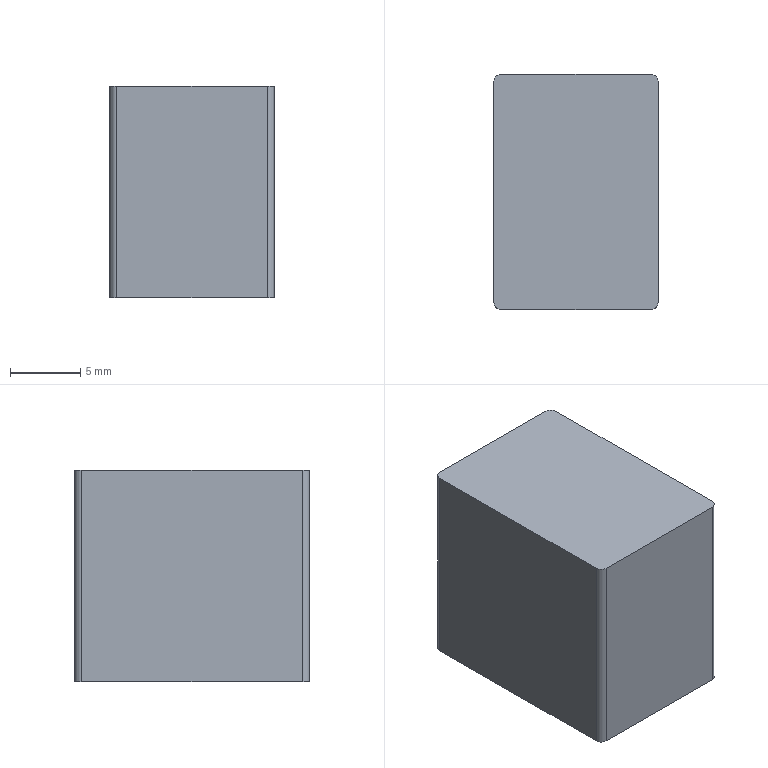Part | NX | features BREP 1 | 1 solid | 10 faces | box 11.656 x 16.683 x 15 mm | volume 2914 mm3 | plane 6 | cylinder 4 | commonest cylinder face diameters 1 x4
STEP:
#1=CARTESIAN_POINT('',(-5.328,8.342,-25.6));
#2=VERTEX_POINT('',#1);
#3=CARTESIAN_POINT('',(-5.828,7.842,-25.6));
#4=VERTEX_POINT('',#3);
#5=CARTESIAN_POINT('',(-5.328,7.842,-25.6));
#6=DIRECTION('',(0.,0.,1.));
#7=DIRECTION('',(1.,0.,0.));
#8=AXIS2_PLACEMENT_3D('',#5,#6,#7);
#9=CIRCLE('',#8,0.5);
#10=EDGE_CURVE('',#2,#4,#9,.T.);
#11=ORIENTED_EDGE('',*,*,#10,.F.);
#12=CARTESIAN_POINT('',(-5.328,8.342,-40.6));
#13=VERTEX_POINT('',#12);
#14=CARTESIAN_POINT('',(-5.328,8.342,-40.6));
#15=DIRECTION('',(0.,0.,1.));
#16=VECTOR('',#15,1000.);
#17=LINE('',#14,#16);
#18=EDGE_CURVE('',#13,#2,#17,.T.);
#19=ORIENTED_EDGE('',*,*,#18,.F.);
#20=CARTESIAN_POINT('',(-5.828,7.842,-40.6));
#21=VERTEX_POINT('',#20);
#22=CARTESIAN_POINT('',(-5.328,7.842,-40.6));
#23=DIRECTION('',(0.,0.,1.));
#24=DIRECTION('',(1.,0.,0.));
#25=AXIS2_PLACEMENT_3D('',#22,#23,#24);
#26=CIRCLE('',#25,0.5);
#27=EDGE_CURVE('',#13,#21,#26,.T.);
#28=ORIENTED_EDGE('',*,*,#27,.T.);
#29=CARTESIAN_POINT('',(-5.828,7.842,-40.6));
#30=DIRECTION('',(0.,0.,1.));
#31=VECTOR('',#30,1000.);
#32=LINE('',#29,#31);
#33=EDGE_CURVE('',#21,#4,#32,.T.);
#34=ORIENTED_EDGE('',*,*,#33,.T.);
#35=EDGE_LOOP('',(#11,#19,#28,#34));
#36=FACE_BOUND('',#35,.T.);
#37=CARTESIAN_POINT('',(-5.328,7.842,-40.6));
#38=DIRECTION('',(0.,0.,1.));
#39=DIRECTION('',(-1.,0.,0.));
#40=AXIS2_PLACEMENT_3D('',#37,#38,#39);
#41=CYLINDRICAL_SURFACE('',#40,0.5);
#42=ADVANCED_FACE('',(#36),#41,.T.);
#43=CARTESIAN_POINT('',(-5.828,-7.842,-25.6));
#44=VERTEX_POINT('',#43);
#45=CARTESIAN_POINT('',(-5.828,-7.842,-25.6));
#46=DIRECTION('',(0.,1.,0.));
#47=VECTOR('',#46,1000.);
#48=LINE('',#45,#47);
#49=EDGE_CURVE('',#44,#4,#48,.T.);
#50=ORIENTED_EDGE('',*,*,#49,.T.);
#51=ORIENTED_EDGE('',*,*,#33,.F.);
#52=CARTESIAN_POINT('',(-5.828,-7.842,-40.6));
#53=VERTEX_POINT('',#52);
#54=CARTESIAN_POINT('',(-5.828,-7.842,-40.6));
#55=DIRECTION('',(0.,1.,0.));
#56=VECTOR('',#55,1000.);
#57=LINE('',#54,#56);
#58=EDGE_CURVE('',#53,#21,#57,.T.);
#59=ORIENTED_EDGE('',*,*,#58,.F.);
#60=CARTESIAN_POINT('',(-5.828,-7.842,-40.6));
#61=DIRECTION('',(0.,0.,1.));
#62=VECTOR('',#61,1000.);
#63=LINE('',#60,#62);
#64=EDGE_CURVE('',#53,#44,#63,.T.);
#65=ORIENTED_EDGE('',*,*,#64,.T.);
#66=EDGE_LOOP('',(#50,#51,#59,#65));
#67=FACE_BOUND('',#66,.T.);
#68=CARTESIAN_POINT('',(-5.828,-7.842,-40.6));
#69=DIRECTION('',(1.,0.,0.));
#70=DIRECTION('',(0.,0.,1.));
#71=AXIS2_PLACEMENT_3D('',#68,#69,#70);
#72=PLANE('',#71);
#73=ADVANCED_FACE('',(#67),#72,.F.);
#74=CARTESIAN_POINT('',(-5.328,-8.342,-25.6));
#75=VERTEX_POINT('',#74);
#76=CARTESIAN_POINT('',(-5.328,-7.842,-25.6));
#77=DIRECTION('',(0.,0.,1.));
#78=DIRECTION('',(1.,0.,0.));
#79=AXIS2_PLACEMENT_3D('',#76,#77,#78);
#80=CIRCLE('',#79,0.5);
#81=EDGE_CURVE('',#44,#75,#80,.T.);
#82=ORIENTED_EDGE('',*,*,#81,.F.);
#83=ORIENTED_EDGE('',*,*,#64,.F.);
#84=CARTESIAN_POINT('',(-5.328,-8.342,-40.6));
#85=VERTEX_POINT('',#84);
#86=CARTESIAN_POINT('',(-5.328,-7.842,-40.6));
#87=DIRECTION('',(0.,0.,1.));
#88=DIRECTION('',(1.,0.,0.));
#89=AXIS2_PLACEMENT_3D('',#86,#87,#88);
#90=CIRCLE('',#89,0.5);
#91=EDGE_CURVE('',#53,#85,#90,.T.);
#92=ORIENTED_EDGE('',*,*,#91,.T.);
#93=CARTESIAN_POINT('',(-5.328,-8.342,-40.6));
#94=DIRECTION('',(0.,0.,1.));
#95=VECTOR('',#94,1000.);
#96=LINE('',#93,#95);
#97=EDGE_CURVE('',#85,#75,#96,.T.);
#98=ORIENTED_EDGE('',*,*,#97,.T.);
#99=EDGE_LOOP('',(#82,#83,#92,#98));
#100=FACE_BOUND('',#99,.T.);
#101=CARTESIAN_POINT('',(-5.328,-7.842,-40.6));
#102=DIRECTION('',(0.,0.,1.));
#103=DIRECTION('',(-1.,0.,0.));
#104=AXIS2_PLACEMENT_3D('',#101,#102,#103);
#105=CYLINDRICAL_SURFACE('',#104,0.5);
#106=ADVANCED_FACE('',(#100),#105,.T.);
#107=CARTESIAN_POINT('',(5.328,-8.342,-25.6));
#108=VERTEX_POINT('',#107);
#109=CARTESIAN_POINT('',(5.328,-8.342,-25.6));
#110=DIRECTION('',(-1.,0.,0.));
#111=VECTOR('',#110,1000.);
#112=LINE('',#109,#111);
#113=EDGE_CURVE('',#108,#75,#112,.T.);
#114=ORIENTED_EDGE('',*,*,#113,.T.);
#115=ORIENTED_EDGE('',*,*,#97,.F.);
#116=CARTESIAN_POINT('',(5.328,-8.342,-40.6));
#117=VERTEX_POINT('',#116);
#118=CARTESIAN_POINT('',(5.328,-8.342,-40.6));
#119=DIRECTION('',(-1.,0.,0.));
#120=VECTOR('',#119,1000.);
#121=LINE('',#118,#120);
#122=EDGE_CURVE('',#117,#85,#121,.T.);
#123=ORIENTED_EDGE('',*,*,#122,.F.);
#124=CARTESIAN_POINT('',(5.328,-8.342,-40.6));
#125=DIRECTION('',(0.,0.,1.));
#126=VECTOR('',#125,1000.);
#127=LINE('',#124,#126);
#128=EDGE_CURVE('',#117,#108,#127,.T.);
#129=ORIENTED_EDGE('',*,*,#128,.T.);
#130=EDGE_LOOP('',(#114,#115,#123,#129));
#131=FACE_BOUND('',#130,.T.);
#132=CARTESIAN_POINT('',(5.328,-8.342,-40.6));
#133=DIRECTION('',(0.,1.,0.));
#134=DIRECTION('',(0.,0.,-1.));
#135=AXIS2_PLACEMENT_3D('',#132,#133,#134);
#136=PLANE('',#135);
#137=ADVANCED_FACE('',(#131),#136,.F.);
#138=CARTESIAN_POINT('',(5.828,-7.842,-25.6));
#139=VERTEX_POINT('',#138);
#140=CARTESIAN_POINT('',(5.328,-7.842,-25.6));
#141=DIRECTION('',(0.,0.,1.));
#142=DIRECTION('',(1.,0.,0.));
#143=AXIS2_PLACEMENT_3D('',#140,#141,#142);
#144=CIRCLE('',#143,0.5);
#145=EDGE_CURVE('',#108,#139,#144,.T.);
#146=ORIENTED_EDGE('',*,*,#145,.F.);
#147=ORIENTED_EDGE('',*,*,#128,.F.);
#148=CARTESIAN_POINT('',(5.828,-7.842,-40.6));
#149=VERTEX_POINT('',#148);
#150=CARTESIAN_POINT('',(5.328,-7.842,-40.6));
#151=DIRECTION('',(0.,0.,1.));
#152=DIRECTION('',(1.,0.,0.));
#153=AXIS2_PLACEMENT_3D('',#150,#151,#152);
#154=CIRCLE('',#153,0.5);
#155=EDGE_CURVE('',#117,#149,#154,.T.);
#156=ORIENTED_EDGE('',*,*,#155,.T.);
#157=CARTESIAN_POINT('',(5.828,-7.842,-40.6));
#158=DIRECTION('',(0.,0.,1.));
#159=VECTOR('',#158,1000.);
#160=LINE('',#157,#159);
#161=EDGE_CURVE('',#149,#139,#160,.T.);
#162=ORIENTED_EDGE('',*,*,#161,.T.);
#163=EDGE_LOOP('',(#146,#147,#156,#162));
#164=FACE_BOUND('',#163,.T.);
#165=CARTESIAN_POINT('',(5.328,-7.842,-40.6));
#166=DIRECTION('',(0.,0.,1.));
#167=DIRECTION('',(-1.,0.,0.));
#168=AXIS2_PLACEMENT_3D('',#165,#166,#167);
#169=CYLINDRICAL_SURFACE('',#168,0.5);
#170=ADVANCED_FACE('',(#164),#169,.T.);
#171=CARTESIAN_POINT('',(5.828,7.842,-25.6));
#172=VERTEX_POINT('',#171);
#173=CARTESIAN_POINT('',(5.828,7.842,-25.6));
#174=DIRECTION('',(0.,-1.,0.));
#175=VECTOR('',#174,1000.);
#176=LINE('',#173,#175);
#177=EDGE_CURVE('',#172,#139,#176,.T.);
#178=ORIENTED_EDGE('',*,*,#177,.T.);
#179=ORIENTED_EDGE('',*,*,#161,.F.);
#180=CARTESIAN_POINT('',(5.828,7.842,-40.6));
#181=VERTEX_POINT('',#180);
#182=CARTESIAN_POINT('',(5.828,7.842,-40.6));
#183=DIRECTION('',(0.,-1.,0.));
#184=VECTOR('',#183,1000.);
#185=LINE('',#182,#184);
#186=EDGE_CURVE('',#181,#149,#185,.T.);
#187=ORIENTED_EDGE('',*,*,#186,.F.);
#188=CARTESIAN_POINT('',(5.828,7.842,-40.6));
#189=DIRECTION('',(0.,0.,1.));
#190=VECTOR('',#189,1000.);
#191=LINE('',#188,#190);
#192=EDGE_CURVE('',#181,#172,#191,.T.);
#193=ORIENTED_EDGE('',*,*,#192,.T.);
#194=EDGE_LOOP('',(#178,#179,#187,#193));
#195=FACE_BOUND('',#194,.T.);
#196=CARTESIAN_POINT('',(5.828,7.842,-40.6));
#197=DIRECTION('',(-1.,0.,0.));
#198=DIRECTION('',(0.,1.,0.));
#199=AXIS2_PLACEMENT_3D('',#196,#197,#198);
#200=PLANE('',#199);
#201=ADVANCED_FACE('',(#195),#200,.F.);
#202=CARTESIAN_POINT('',(5.328,8.342,-25.6));
#203=VERTEX_POINT('',#202);
#204=CARTESIAN_POINT('',(5.328,7.842,-25.6));
#205=DIRECTION('',(0.,0.,1.));
#206=DIRECTION('',(1.,0.,0.));
#207=AXIS2_PLACEMENT_3D('',#204,#205,#206);
#208=CIRCLE('',#207,0.5);
#209=EDGE_CURVE('',#172,#203,#208,.T.);
#210=ORIENTED_EDGE('',*,*,#209,.F.);
#211=ORIENTED_EDGE('',*,*,#192,.F.);
#212=CARTESIAN_POINT('',(5.328,8.342,-40.6));
#213=VERTEX_POINT('',#212);
#214=CARTESIAN_POINT('',(5.328,7.842,-40.6));
#215=DIRECTION('',(0.,0.,1.));
#216=DIRECTION('',(1.,0.,0.));
#217=AXIS2_PLACEMENT_3D('',#214,#215,#216);
#218=CIRCLE('',#217,0.5);
#219=EDGE_CURVE('',#181,#213,#218,.T.);
#220=ORIENTED_EDGE('',*,*,#219,.T.);
#221=CARTESIAN_POINT('',(5.328,8.342,-40.6));
#222=DIRECTION('',(0.,0.,1.));
#223=VECTOR('',#222,1000.);
#224=LINE('',#221,#223);
#225=EDGE_CURVE('',#213,#203,#224,.T.);
#226=ORIENTED_EDGE('',*,*,#225,.T.);
#227=EDGE_LOOP('',(#210,#211,#220,#226));
#228=FACE_BOUND('',#227,.T.);
#229=CARTESIAN_POINT('',(5.328,7.842,-40.6));
#230=DIRECTION('',(0.,0.,1.));
#231=DIRECTION('',(-1.,0.,0.));
#232=AXIS2_PLACEMENT_3D('',#229,#230,#231);
#233=CYLINDRICAL_SURFACE('',#232,0.5);
#234=ADVANCED_FACE('',(#228),#233,.T.);
#235=CARTESIAN_POINT('',(-5.328,8.342,-25.6));
#236=DIRECTION('',(1.,0.,0.));
#237=VECTOR('',#236,1000.);
#238=LINE('',#235,#237);
#239=EDGE_CURVE('',#2,#203,#238,.T.);
#240=ORIENTED_EDGE('',*,*,#239,.T.);
#241=ORIENTED_EDGE('',*,*,#225,.F.);
#242=CARTESIAN_POINT('',(-5.328,8.342,-40.6));
#243=DIRECTION('',(1.,0.,0.));
#244=VECTOR('',#243,1000.);
#245=LINE('',#242,#244);
#246=EDGE_CURVE('',#13,#213,#245,.T.);
#247=ORIENTED_EDGE('',*,*,#246,.F.);
#248=ORIENTED_EDGE('',*,*,#18,.T.);
#249=EDGE_LOOP('',(#240,#241,#247,#248));
#250=FACE_BOUND('',#249,.T.);
#251=CARTESIAN_POINT('',(-5.328,8.342,-40.6));
#252=DIRECTION('',(0.,-1.,0.));
#253=DIRECTION('',(0.,0.,1.));
#254=AXIS2_PLACEMENT_3D('',#251,#252,#253);
#255=PLANE('',#254);
#256=ADVANCED_FACE('',(#250),#255,.F.);
#257=ORIENTED_EDGE('',*,*,#27,.F.);
#258=ORIENTED_EDGE('',*,*,#246,.T.);
#259=ORIENTED_EDGE('',*,*,#219,.F.);
#260=ORIENTED_EDGE('',*,*,#186,.T.);
#261=ORIENTED_EDGE('',*,*,#155,.F.);
#262=ORIENTED_EDGE('',*,*,#122,.T.);
#263=ORIENTED_EDGE('',*,*,#91,.F.);
#264=ORIENTED_EDGE('',*,*,#58,.T.);
#265=EDGE_LOOP('',(#257,#258,#259,#260,#261,#262,#263,#264));
#266=FACE_BOUND('',#265,.T.);
#267=CARTESIAN_POINT('',(-5.328,7.842,-40.6));
#268=DIRECTION('',(0.,0.,1.));
#269=DIRECTION('',(-1.,0.,0.));
#270=AXIS2_PLACEMENT_3D('',#267,#268,#269);
#271=PLANE('',#270);
#272=ADVANCED_FACE('',(#266),#271,.F.);
#273=ORIENTED_EDGE('',*,*,#10,.T.);
#274=ORIENTED_EDGE('',*,*,#49,.F.);
#275=ORIENTED_EDGE('',*,*,#81,.T.);
#276=ORIENTED_EDGE('',*,*,#113,.F.);
#277=ORIENTED_EDGE('',*,*,#145,.T.);
#278=ORIENTED_EDGE('',*,*,#177,.F.);
#279=ORIENTED_EDGE('',*,*,#209,.T.);
#280=ORIENTED_EDGE('',*,*,#239,.F.);
#281=EDGE_LOOP('',(#273,#274,#275,#276,#277,#278,#279,#280));
#282=FACE_BOUND('',#281,.T.);
#283=CARTESIAN_POINT('',(-5.328,7.842,-25.6));
#284=DIRECTION('',(0.,0.,1.));
#285=DIRECTION('',(-1.,0.,0.));
#286=AXIS2_PLACEMENT_3D('',#283,#284,#285);
#287=PLANE('',#286);
#288=ADVANCED_FACE('',(#282),#287,.T.);
#289=CLOSED_SHELL('',(#42,#73,#106,#137,#170,#201,#234,#256,#272,#288));
#290=MANIFOLD_SOLID_BREP('',#289);
#291=(LENGTH_UNIT()NAMED_UNIT(*)SI_UNIT(.MILLI.,.METRE.));
#292=UNCERTAINTY_MEASURE_WITH_UNIT(LENGTH_MEASURE(0.00001),#291,'','');
#293=(NAMED_UNIT(*)PLANE_ANGLE_UNIT()SI_UNIT($,.RADIAN.));
#294=(NAMED_UNIT(*)SI_UNIT($,.STERADIAN.)SOLID_ANGLE_UNIT());
#295=(GEOMETRIC_REPRESENTATION_CONTEXT(3)GLOBAL_UNCERTAINTY_ASSIGNED_CONTEXT((#292))GLOBAL_UNIT_ASSIGNED_CONTEXT((#291,#293,#294))REPRESENTATION_CONTEXT('',''));
#296=ADVANCED_BREP_SHAPE_REPRESENTATION('',(#290),#295);